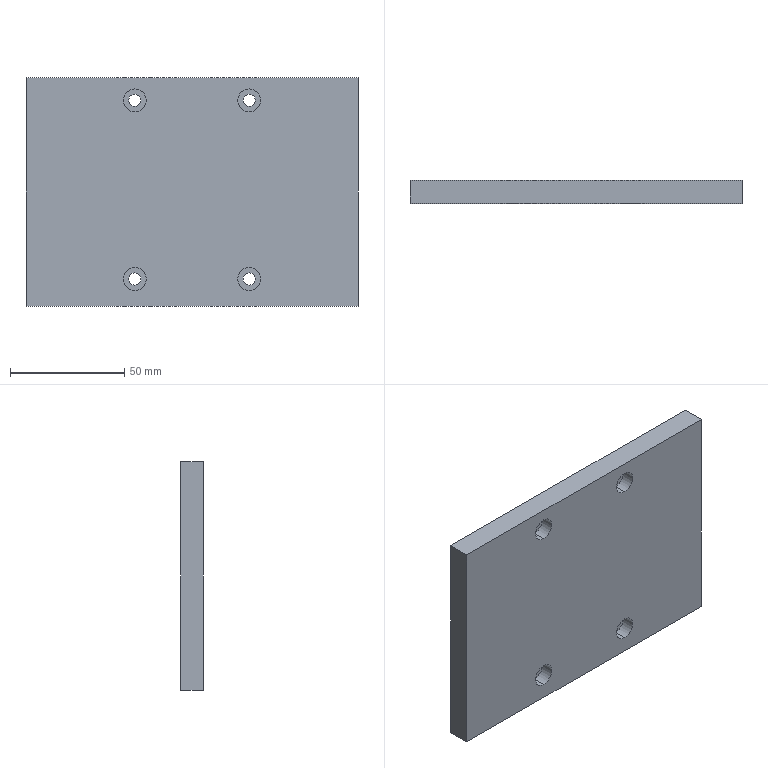Part | SolidWorks | features BaseBody 1 | 1 solid | 26 faces | box 145 x 10 x 100 mm | volume 142830 mm3 | cylinder 16 | plane 10 | commonest cylinder face diameters 5.3 x8 10 x8
STEP:
#1=CARTESIAN_POINT('',(-152.496,1790.044,-108.85));
#2=VERTEX_POINT('',#1);
#3=CARTESIAN_POINT('',(-152.496,1790.044,-114.15));
#4=VERTEX_POINT('',#3);
#5=CARTESIAN_POINT('',(-152.496,1790.044,-111.5));
#6=DIRECTION('',(0.,-1.,0.));
#7=DIRECTION('',(0.,0.,-1.));
#8=AXIS2_PLACEMENT_3D('',#5,#6,#7);
#9=CIRCLE('',#8,2.65);
#10=EDGE_CURVE('',#2,#4,#9,.T.);
#11=ORIENTED_EDGE('',*,*,#10,.F.);
#12=CARTESIAN_POINT('',(-152.496,1785.744,-108.85));
#13=VERTEX_POINT('',#12);
#14=CARTESIAN_POINT('',(-152.496,1780.044,-108.85));
#15=DIRECTION('',(0.,-1.,0.));
#16=VECTOR('',#15,1000.);
#17=LINE('',#14,#16);
#18=EDGE_CURVE('',#2,#13,#17,.T.);
#19=ORIENTED_EDGE('',*,*,#18,.T.);
#20=CARTESIAN_POINT('',(-152.496,1785.744,-114.15));
#21=VERTEX_POINT('',#20);
#22=CARTESIAN_POINT('',(-152.496,1785.744,-111.5));
#23=DIRECTION('',(0.,1.,0.));
#24=DIRECTION('',(0.,0.,-1.));
#25=AXIS2_PLACEMENT_3D('',#22,#23,#24);
#26=CIRCLE('',#25,2.65);
#27=EDGE_CURVE('',#21,#13,#26,.T.);
#28=ORIENTED_EDGE('',*,*,#27,.F.);
#29=CARTESIAN_POINT('',(-152.496,1780.044,-114.15));
#30=DIRECTION('',(0.,-1.,0.));
#31=VECTOR('',#30,1000.);
#32=LINE('',#29,#31);
#33=EDGE_CURVE('',#4,#21,#32,.T.);
#34=ORIENTED_EDGE('',*,*,#33,.F.);
#35=EDGE_LOOP('',(#11,#19,#28,#34));
#36=FACE_OUTER_BOUND('',#35,.T.);
#37=CARTESIAN_POINT('',(-152.496,1780.044,-111.5));
#38=DIRECTION('',(0.,-1.,0.));
#39=DIRECTION('',(0.,0.,-1.));
#40=AXIS2_PLACEMENT_3D('',#37,#38,#39);
#41=CYLINDRICAL_SURFACE('',#40,2.65);
#42=ADVANCED_FACE('',(#36),#41,.F.);
#43=CARTESIAN_POINT('',(-152.496,1790.044,-30.85));
#44=VERTEX_POINT('',#43);
#45=CARTESIAN_POINT('',(-152.496,1790.044,-36.15));
#46=VERTEX_POINT('',#45);
#47=CARTESIAN_POINT('',(-152.496,1790.044,-33.5));
#48=DIRECTION('',(0.,-1.,0.));
#49=DIRECTION('',(0.,0.,-1.));
#50=AXIS2_PLACEMENT_3D('',#47,#48,#49);
#51=CIRCLE('',#50,2.65);
#52=EDGE_CURVE('',#44,#46,#51,.T.);
#53=ORIENTED_EDGE('',*,*,#52,.F.);
#54=CARTESIAN_POINT('',(-152.496,1785.744,-30.85));
#55=VERTEX_POINT('',#54);
#56=CARTESIAN_POINT('',(-152.496,1780.044,-30.85));
#57=DIRECTION('',(0.,-1.,0.));
#58=VECTOR('',#57,1000.);
#59=LINE('',#56,#58);
#60=EDGE_CURVE('',#44,#55,#59,.T.);
#61=ORIENTED_EDGE('',*,*,#60,.T.);
#62=CARTESIAN_POINT('',(-152.496,1785.744,-36.15));
#63=VERTEX_POINT('',#62);
#64=CARTESIAN_POINT('',(-152.496,1785.744,-33.5));
#65=DIRECTION('',(0.,1.,0.));
#66=DIRECTION('',(0.,0.,-1.));
#67=AXIS2_PLACEMENT_3D('',#64,#65,#66);
#68=CIRCLE('',#67,2.65);
#69=EDGE_CURVE('',#63,#55,#68,.T.);
#70=ORIENTED_EDGE('',*,*,#69,.F.);
#71=CARTESIAN_POINT('',(-152.496,1780.044,-36.15));
#72=DIRECTION('',(0.,-1.,0.));
#73=VECTOR('',#72,1000.);
#74=LINE('',#71,#73);
#75=EDGE_CURVE('',#46,#63,#74,.T.);
#76=ORIENTED_EDGE('',*,*,#75,.F.);
#77=EDGE_LOOP('',(#53,#61,#70,#76));
#78=FACE_OUTER_BOUND('',#77,.T.);
#79=CARTESIAN_POINT('',(-152.496,1780.044,-33.5));
#80=DIRECTION('',(0.,-1.,0.));
#81=DIRECTION('',(0.,0.,-1.));
#82=AXIS2_PLACEMENT_3D('',#79,#80,#81);
#83=CYLINDRICAL_SURFACE('',#82,2.65);
#84=ADVANCED_FACE('',(#78),#83,.F.);
#85=CARTESIAN_POINT('',(-102.496,1790.044,-30.85));
#86=VERTEX_POINT('',#85);
#87=CARTESIAN_POINT('',(-102.496,1790.044,-36.15));
#88=VERTEX_POINT('',#87);
#89=CARTESIAN_POINT('',(-102.496,1790.044,-33.5));
#90=DIRECTION('',(0.,-1.,0.));
#91=DIRECTION('',(0.,0.,-1.));
#92=AXIS2_PLACEMENT_3D('',#89,#90,#91);
#93=CIRCLE('',#92,2.65);
#94=EDGE_CURVE('',#86,#88,#93,.T.);
#95=ORIENTED_EDGE('',*,*,#94,.F.);
#96=CARTESIAN_POINT('',(-102.496,1785.744,-30.85));
#97=VERTEX_POINT('',#96);
#98=CARTESIAN_POINT('',(-102.496,1780.044,-30.85));
#99=DIRECTION('',(0.,-1.,0.));
#100=VECTOR('',#99,1000.);
#101=LINE('',#98,#100);
#102=EDGE_CURVE('',#86,#97,#101,.T.);
#103=ORIENTED_EDGE('',*,*,#102,.T.);
#104=CARTESIAN_POINT('',(-102.496,1785.744,-36.15));
#105=VERTEX_POINT('',#104);
#106=CARTESIAN_POINT('',(-102.496,1785.744,-33.5));
#107=DIRECTION('',(0.,1.,0.));
#108=DIRECTION('',(0.,0.,-1.));
#109=AXIS2_PLACEMENT_3D('',#106,#107,#108);
#110=CIRCLE('',#109,2.65);
#111=EDGE_CURVE('',#105,#97,#110,.T.);
#112=ORIENTED_EDGE('',*,*,#111,.F.);
#113=CARTESIAN_POINT('',(-102.496,1780.044,-36.15));
#114=DIRECTION('',(0.,-1.,0.));
#115=VECTOR('',#114,1000.);
#116=LINE('',#113,#115);
#117=EDGE_CURVE('',#88,#105,#116,.T.);
#118=ORIENTED_EDGE('',*,*,#117,.F.);
#119=EDGE_LOOP('',(#95,#103,#112,#118));
#120=FACE_OUTER_BOUND('',#119,.T.);
#121=CARTESIAN_POINT('',(-102.496,1780.044,-33.5));
#122=DIRECTION('',(0.,-1.,0.));
#123=DIRECTION('',(0.,0.,-1.));
#124=AXIS2_PLACEMENT_3D('',#121,#122,#123);
#125=CYLINDRICAL_SURFACE('',#124,2.65);
#126=ADVANCED_FACE('',(#120),#125,.F.);
#127=CARTESIAN_POINT('',(-102.496,1790.044,-108.85));
#128=VERTEX_POINT('',#127);
#129=CARTESIAN_POINT('',(-102.496,1790.044,-114.15));
#130=VERTEX_POINT('',#129);
#131=CARTESIAN_POINT('',(-102.496,1790.044,-111.5));
#132=DIRECTION('',(0.,-1.,0.));
#133=DIRECTION('',(0.,0.,-1.));
#134=AXIS2_PLACEMENT_3D('',#131,#132,#133);
#135=CIRCLE('',#134,2.65);
#136=EDGE_CURVE('',#128,#130,#135,.T.);
#137=ORIENTED_EDGE('',*,*,#136,.F.);
#138=CARTESIAN_POINT('',(-102.496,1785.744,-108.85));
#139=VERTEX_POINT('',#138);
#140=CARTESIAN_POINT('',(-102.496,1780.044,-108.85));
#141=DIRECTION('',(0.,-1.,0.));
#142=VECTOR('',#141,1000.);
#143=LINE('',#140,#142);
#144=EDGE_CURVE('',#128,#139,#143,.T.);
#145=ORIENTED_EDGE('',*,*,#144,.T.);
#146=CARTESIAN_POINT('',(-102.496,1785.744,-114.15));
#147=VERTEX_POINT('',#146);
#148=CARTESIAN_POINT('',(-102.496,1785.744,-111.5));
#149=DIRECTION('',(0.,1.,0.));
#150=DIRECTION('',(0.,0.,-1.));
#151=AXIS2_PLACEMENT_3D('',#148,#149,#150);
#152=CIRCLE('',#151,2.65);
#153=EDGE_CURVE('',#147,#139,#152,.T.);
#154=ORIENTED_EDGE('',*,*,#153,.F.);
#155=CARTESIAN_POINT('',(-102.496,1780.044,-114.15));
#156=DIRECTION('',(0.,-1.,0.));
#157=VECTOR('',#156,1000.);
#158=LINE('',#155,#157);
#159=EDGE_CURVE('',#130,#147,#158,.T.);
#160=ORIENTED_EDGE('',*,*,#159,.F.);
#161=EDGE_LOOP('',(#137,#145,#154,#160));
#162=FACE_OUTER_BOUND('',#161,.T.);
#163=CARTESIAN_POINT('',(-102.496,1780.044,-111.5));
#164=DIRECTION('',(0.,-1.,0.));
#165=DIRECTION('',(0.,0.,-1.));
#166=AXIS2_PLACEMENT_3D('',#163,#164,#165);
#167=CYLINDRICAL_SURFACE('',#166,2.65);
#168=ADVANCED_FACE('',(#162),#167,.F.);
#169=CARTESIAN_POINT('',(-152.496,1785.744,-116.5));
#170=VERTEX_POINT('',#169);
#171=CARTESIAN_POINT('',(-152.496,1785.744,-106.5));
#172=VERTEX_POINT('',#171);
#173=CARTESIAN_POINT('',(-152.496,1785.744,-111.5));
#174=DIRECTION('',(0.,1.,0.));
#175=DIRECTION('',(0.,0.,-1.));
#176=AXIS2_PLACEMENT_3D('',#173,#174,#175);
#177=CIRCLE('',#176,5.);
#178=EDGE_CURVE('',#170,#172,#177,.T.);
#179=ORIENTED_EDGE('',*,*,#178,.T.);
#180=CARTESIAN_POINT('',(-152.496,1780.044,-106.5));
#181=VERTEX_POINT('',#180);
#182=CARTESIAN_POINT('',(-152.496,1780.044,-106.5));
#183=DIRECTION('',(0.,-1.,0.));
#184=VECTOR('',#183,1000.);
#185=LINE('',#182,#184);
#186=EDGE_CURVE('',#172,#181,#185,.T.);
#187=ORIENTED_EDGE('',*,*,#186,.T.);
#188=CARTESIAN_POINT('',(-152.496,1780.044,-116.5));
#189=VERTEX_POINT('',#188);
#190=CARTESIAN_POINT('',(-152.496,1780.044,-111.5));
#191=DIRECTION('',(0.,-1.,0.));
#192=DIRECTION('',(0.,0.,-1.));
#193=AXIS2_PLACEMENT_3D('',#190,#191,#192);
#194=CIRCLE('',#193,5.);
#195=EDGE_CURVE('',#181,#189,#194,.T.);
#196=ORIENTED_EDGE('',*,*,#195,.T.);
#197=CARTESIAN_POINT('',(-152.496,1780.044,-116.5));
#198=DIRECTION('',(0.,-1.,0.));
#199=VECTOR('',#198,1000.);
#200=LINE('',#197,#199);
#201=EDGE_CURVE('',#170,#189,#200,.T.);
#202=ORIENTED_EDGE('',*,*,#201,.F.);
#203=EDGE_LOOP('',(#179,#187,#196,#202));
#204=FACE_OUTER_BOUND('',#203,.T.);
#205=CARTESIAN_POINT('',(-152.496,1780.044,-111.5));
#206=DIRECTION('',(0.,-1.,0.));
#207=DIRECTION('',(0.,0.,-1.));
#208=AXIS2_PLACEMENT_3D('',#205,#206,#207);
#209=CYLINDRICAL_SURFACE('',#208,5.);
#210=ADVANCED_FACE('',(#204),#209,.F.);
#211=CARTESIAN_POINT('',(-152.496,1785.744,-38.5));
#212=VERTEX_POINT('',#211);
#213=CARTESIAN_POINT('',(-152.496,1785.744,-28.5));
#214=VERTEX_POINT('',#213);
#215=CARTESIAN_POINT('',(-152.496,1785.744,-33.5));
#216=DIRECTION('',(0.,1.,0.));
#217=DIRECTION('',(0.,0.,-1.));
#218=AXIS2_PLACEMENT_3D('',#215,#216,#217);
#219=CIRCLE('',#218,5.);
#220=EDGE_CURVE('',#212,#214,#219,.T.);
#221=ORIENTED_EDGE('',*,*,#220,.T.);
#222=CARTESIAN_POINT('',(-152.496,1780.044,-28.5));
#223=VERTEX_POINT('',#222);
#224=CARTESIAN_POINT('',(-152.496,1780.044,-28.5));
#225=DIRECTION('',(0.,-1.,0.));
#226=VECTOR('',#225,1000.);
#227=LINE('',#224,#226);
#228=EDGE_CURVE('',#214,#223,#227,.T.);
#229=ORIENTED_EDGE('',*,*,#228,.T.);
#230=CARTESIAN_POINT('',(-152.496,1780.044,-38.5));
#231=VERTEX_POINT('',#230);
#232=CARTESIAN_POINT('',(-152.496,1780.044,-33.5));
#233=DIRECTION('',(0.,-1.,0.));
#234=DIRECTION('',(0.,0.,-1.));
#235=AXIS2_PLACEMENT_3D('',#232,#233,#234);
#236=CIRCLE('',#235,5.);
#237=EDGE_CURVE('',#223,#231,#236,.T.);
#238=ORIENTED_EDGE('',*,*,#237,.T.);
#239=CARTESIAN_POINT('',(-152.496,1780.044,-38.5));
#240=DIRECTION('',(0.,-1.,0.));
#241=VECTOR('',#240,1000.);
#242=LINE('',#239,#241);
#243=EDGE_CURVE('',#212,#231,#242,.T.);
#244=ORIENTED_EDGE('',*,*,#243,.F.);
#245=EDGE_LOOP('',(#221,#229,#238,#244));
#246=FACE_OUTER_BOUND('',#245,.T.);
#247=CARTESIAN_POINT('',(-152.496,1780.044,-33.5));
#248=DIRECTION('',(0.,-1.,0.));
#249=DIRECTION('',(0.,0.,-1.));
#250=AXIS2_PLACEMENT_3D('',#247,#248,#249);
#251=CYLINDRICAL_SURFACE('',#250,5.);
#252=ADVANCED_FACE('',(#246),#251,.F.);
#253=CARTESIAN_POINT('',(-102.496,1785.744,-38.5));
#254=VERTEX_POINT('',#253);
#255=CARTESIAN_POINT('',(-102.496,1785.744,-28.5));
#256=VERTEX_POINT('',#255);
#257=CARTESIAN_POINT('',(-102.496,1785.744,-33.5));
#258=DIRECTION('',(0.,1.,0.));
#259=DIRECTION('',(0.,0.,-1.));
#260=AXIS2_PLACEMENT_3D('',#257,#258,#259);
#261=CIRCLE('',#260,5.);
#262=EDGE_CURVE('',#254,#256,#261,.T.);
#263=ORIENTED_EDGE('',*,*,#262,.T.);
#264=CARTESIAN_POINT('',(-102.496,1780.044,-28.5));
#265=VERTEX_POINT('',#264);
#266=CARTESIAN_POINT('',(-102.496,1780.044,-28.5));
#267=DIRECTION('',(0.,-1.,0.));
#268=VECTOR('',#267,1000.);
#269=LINE('',#266,#268);
#270=EDGE_CURVE('',#256,#265,#269,.T.);
#271=ORIENTED_EDGE('',*,*,#270,.T.);
#272=CARTESIAN_POINT('',(-102.496,1780.044,-38.5));
#273=VERTEX_POINT('',#272);
#274=CARTESIAN_POINT('',(-102.496,1780.044,-33.5));
#275=DIRECTION('',(0.,-1.,0.));
#276=DIRECTION('',(0.,0.,-1.));
#277=AXIS2_PLACEMENT_3D('',#274,#275,#276);
#278=CIRCLE('',#277,5.);
#279=EDGE_CURVE('',#265,#273,#278,.T.);
#280=ORIENTED_EDGE('',*,*,#279,.T.);
#281=CARTESIAN_POINT('',(-102.496,1780.044,-38.5));
#282=DIRECTION('',(0.,-1.,0.));
#283=VECTOR('',#282,1000.);
#284=LINE('',#281,#283);
#285=EDGE_CURVE('',#254,#273,#284,.T.);
#286=ORIENTED_EDGE('',*,*,#285,.F.);
#287=EDGE_LOOP('',(#263,#271,#280,#286));
#288=FACE_OUTER_BOUND('',#287,.T.);
#289=CARTESIAN_POINT('',(-102.496,1780.044,-33.5));
#290=DIRECTION('',(0.,-1.,0.));
#291=DIRECTION('',(0.,0.,-1.));
#292=AXIS2_PLACEMENT_3D('',#289,#290,#291);
#293=CYLINDRICAL_SURFACE('',#292,5.);
#294=ADVANCED_FACE('',(#288),#293,.F.);
#295=CARTESIAN_POINT('',(-102.496,1785.744,-116.5));
#296=VERTEX_POINT('',#295);
#297=CARTESIAN_POINT('',(-102.496,1785.744,-106.5));
#298=VERTEX_POINT('',#297);
#299=CARTESIAN_POINT('',(-102.496,1785.744,-111.5));
#300=DIRECTION('',(0.,1.,0.));
#301=DIRECTION('',(0.,0.,-1.));
#302=AXIS2_PLACEMENT_3D('',#299,#300,#301);
#303=CIRCLE('',#302,5.);
#304=EDGE_CURVE('',#296,#298,#303,.T.);
#305=ORIENTED_EDGE('',*,*,#304,.T.);
#306=CARTESIAN_POINT('',(-102.496,1780.044,-106.5));
#307=VERTEX_POINT('',#306);
#308=CARTESIAN_POINT('',(-102.496,1780.044,-106.5));
#309=DIRECTION('',(0.,-1.,0.));
#310=VECTOR('',#309,1000.);
#311=LINE('',#308,#310);
#312=EDGE_CURVE('',#298,#307,#311,.T.);
#313=ORIENTED_EDGE('',*,*,#312,.T.);
#314=CARTESIAN_POINT('',(-102.496,1780.044,-116.5));
#315=VERTEX_POINT('',#314);
#316=CARTESIAN_POINT('',(-102.496,1780.044,-111.5));
#317=DIRECTION('',(0.,-1.,0.));
#318=DIRECTION('',(0.,0.,-1.));
#319=AXIS2_PLACEMENT_3D('',#316,#317,#318);
#320=CIRCLE('',#319,5.);
#321=EDGE_CURVE('',#307,#315,#320,.T.);
#322=ORIENTED_EDGE('',*,*,#321,.T.);
#323=CARTESIAN_POINT('',(-102.496,1780.044,-116.5));
#324=DIRECTION('',(0.,-1.,0.));
#325=VECTOR('',#324,1000.);
#326=LINE('',#323,#325);
#327=EDGE_CURVE('',#296,#315,#326,.T.);
#328=ORIENTED_EDGE('',*,*,#327,.F.);
#329=EDGE_LOOP('',(#305,#313,#322,#328));
#330=FACE_OUTER_BOUND('',#329,.T.);
#331=CARTESIAN_POINT('',(-102.496,1780.044,-111.5));
#332=DIRECTION('',(0.,-1.,0.));
#333=DIRECTION('',(0.,0.,-1.));
#334=AXIS2_PLACEMENT_3D('',#331,#332,#333);
#335=CYLINDRICAL_SURFACE('',#334,5.);
#336=ADVANCED_FACE('',(#330),#335,.F.);
#337=CARTESIAN_POINT('',(-152.496,1790.044,-111.5));
#338=DIRECTION('',(0.,-1.,0.));
#339=DIRECTION('',(0.,0.,-1.));
#340=AXIS2_PLACEMENT_3D('',#337,#338,#339);
#341=CIRCLE('',#340,2.65);
#342=EDGE_CURVE('',#4,#2,#341,.T.);
#343=ORIENTED_EDGE('',*,*,#342,.T.);
#344=ORIENTED_EDGE('',*,*,#10,.T.);
#345=EDGE_LOOP('',(#343,#344));
#346=FACE_BOUND('',#345,.T.);
#347=CARTESIAN_POINT('',(-152.496,1790.044,-33.5));
#348=DIRECTION('',(0.,-1.,0.));
#349=DIRECTION('',(0.,0.,-1.));
#350=AXIS2_PLACEMENT_3D('',#347,#348,#349);
#351=CIRCLE('',#350,2.65);
#352=EDGE_CURVE('',#46,#44,#351,.T.);
#353=ORIENTED_EDGE('',*,*,#352,.T.);
#354=ORIENTED_EDGE('',*,*,#52,.T.);
#355=EDGE_LOOP('',(#353,#354));
#356=FACE_BOUND('',#355,.T.);
#357=CARTESIAN_POINT('',(-102.496,1790.044,-33.5));
#358=DIRECTION('',(0.,-1.,0.));
#359=DIRECTION('',(0.,0.,-1.));
#360=AXIS2_PLACEMENT_3D('',#357,#358,#359);
#361=CIRCLE('',#360,2.65);
#362=EDGE_CURVE('',#88,#86,#361,.T.);
#363=ORIENTED_EDGE('',*,*,#362,.T.);
#364=ORIENTED_EDGE('',*,*,#94,.T.);
#365=EDGE_LOOP('',(#363,#364));
#366=FACE_BOUND('',#365,.T.);
#367=CARTESIAN_POINT('',(-102.496,1790.044,-111.5));
#368=DIRECTION('',(0.,-1.,0.));
#369=DIRECTION('',(0.,0.,-1.));
#370=AXIS2_PLACEMENT_3D('',#367,#368,#369);
#371=CIRCLE('',#370,2.65);
#372=EDGE_CURVE('',#130,#128,#371,.T.);
#373=ORIENTED_EDGE('',*,*,#372,.T.);
#374=ORIENTED_EDGE('',*,*,#136,.T.);
#375=EDGE_LOOP('',(#373,#374));
#376=FACE_BOUND('',#375,.T.);
#377=CARTESIAN_POINT('',(-199.996,1790.044,-123.5));
#378=VERTEX_POINT('',#377);
#379=CARTESIAN_POINT('',(-199.996,1790.044,-23.5));
#380=VERTEX_POINT('',#379);
#381=CARTESIAN_POINT('',(-199.996,1790.044,-123.5));
#382=DIRECTION('',(0.,0.,1.));
#383=VECTOR('',#382,1000.);
#384=LINE('',#381,#383);
#385=EDGE_CURVE('',#378,#380,#384,.T.);
#386=ORIENTED_EDGE('',*,*,#385,.T.);
#387=CARTESIAN_POINT('',(-54.996,1790.044,-23.5));
#388=VERTEX_POINT('',#387);
#389=CARTESIAN_POINT('',(47.504,1790.044,-23.5));
#390=DIRECTION('',(1.,0.,0.));
#391=VECTOR('',#390,1000.);
#392=LINE('',#389,#391);
#393=EDGE_CURVE('',#380,#388,#392,.T.);
#394=ORIENTED_EDGE('',*,*,#393,.T.);
#395=CARTESIAN_POINT('',(-54.996,1790.044,-123.5));
#396=VERTEX_POINT('',#395);
#397=CARTESIAN_POINT('',(-54.996,1790.044,-123.5));
#398=DIRECTION('',(0.,0.,-1.));
#399=VECTOR('',#398,1000.);
#400=LINE('',#397,#399);
#401=EDGE_CURVE('',#388,#396,#400,.T.);
#402=ORIENTED_EDGE('',*,*,#401,.T.);
#403=CARTESIAN_POINT('',(47.504,1790.044,-123.5));
#404=DIRECTION('',(-1.,0.,0.));
#405=VECTOR('',#404,1000.);
#406=LINE('',#403,#405);
#407=EDGE_CURVE('',#396,#378,#406,.T.);
#408=ORIENTED_EDGE('',*,*,#407,.T.);
#409=EDGE_LOOP('',(#386,#394,#402,#408));
#410=FACE_OUTER_BOUND('',#409,.T.);
#411=CARTESIAN_POINT('',(47.504,1790.044,-123.5));
#412=DIRECTION('',(0.,1.,0.));
#413=DIRECTION('',(0.,0.,1.));
#414=AXIS2_PLACEMENT_3D('',#411,#412,#413);
#415=PLANE('',#414);
#416=ADVANCED_FACE('',(#346,#356,#366,#376,#410),#415,.T.);
#417=ORIENTED_EDGE('',*,*,#18,.F.);
#418=ORIENTED_EDGE('',*,*,#342,.F.);
#419=ORIENTED_EDGE('',*,*,#33,.T.);
#420=CARTESIAN_POINT('',(-152.496,1785.744,-111.5));
#421=DIRECTION('',(0.,1.,0.));
#422=DIRECTION('',(0.,0.,-1.));
#423=AXIS2_PLACEMENT_3D('',#420,#421,#422);
#424=CIRCLE('',#423,2.65);
#425=EDGE_CURVE('',#13,#21,#424,.T.);
#426=ORIENTED_EDGE('',*,*,#425,.F.);
#427=EDGE_LOOP('',(#417,#418,#419,#426));
#428=FACE_OUTER_BOUND('',#427,.T.);
#429=CARTESIAN_POINT('',(-152.496,1780.044,-111.5));
#430=DIRECTION('',(0.,-1.,0.));
#431=DIRECTION('',(0.,0.,-1.));
#432=AXIS2_PLACEMENT_3D('',#429,#430,#431);
#433=CYLINDRICAL_SURFACE('',#432,2.65);
#434=ADVANCED_FACE('',(#428),#433,.F.);
#435=ORIENTED_EDGE('',*,*,#60,.F.);
#436=ORIENTED_EDGE('',*,*,#352,.F.);
#437=ORIENTED_EDGE('',*,*,#75,.T.);
#438=CARTESIAN_POINT('',(-152.496,1785.744,-33.5));
#439=DIRECTION('',(0.,1.,0.));
#440=DIRECTION('',(0.,0.,-1.));
#441=AXIS2_PLACEMENT_3D('',#438,#439,#440);
#442=CIRCLE('',#441,2.65);
#443=EDGE_CURVE('',#55,#63,#442,.T.);
#444=ORIENTED_EDGE('',*,*,#443,.F.);
#445=EDGE_LOOP('',(#435,#436,#437,#444));
#446=FACE_OUTER_BOUND('',#445,.T.);
#447=CARTESIAN_POINT('',(-152.496,1780.044,-33.5));
#448=DIRECTION('',(0.,-1.,0.));
#449=DIRECTION('',(0.,0.,-1.));
#450=AXIS2_PLACEMENT_3D('',#447,#448,#449);
#451=CYLINDRICAL_SURFACE('',#450,2.65);
#452=ADVANCED_FACE('',(#446),#451,.F.);
#453=ORIENTED_EDGE('',*,*,#102,.F.);
#454=ORIENTED_EDGE('',*,*,#362,.F.);
#455=ORIENTED_EDGE('',*,*,#117,.T.);
#456=CARTESIAN_POINT('',(-102.496,1785.744,-33.5));
#457=DIRECTION('',(0.,1.,0.));
#458=DIRECTION('',(0.,0.,-1.));
#459=AXIS2_PLACEMENT_3D('',#456,#457,#458);
#460=CIRCLE('',#459,2.65);
#461=EDGE_CURVE('',#97,#105,#460,.T.);
#462=ORIENTED_EDGE('',*,*,#461,.F.);
#463=EDGE_LOOP('',(#453,#454,#455,#462));
#464=FACE_OUTER_BOUND('',#463,.T.);
#465=CARTESIAN_POINT('',(-102.496,1780.044,-33.5));
#466=DIRECTION('',(0.,-1.,0.));
#467=DIRECTION('',(0.,0.,-1.));
#468=AXIS2_PLACEMENT_3D('',#465,#466,#467);
#469=CYLINDRICAL_SURFACE('',#468,2.65);
#470=ADVANCED_FACE('',(#464),#469,.F.);
#471=ORIENTED_EDGE('',*,*,#144,.F.);
#472=ORIENTED_EDGE('',*,*,#372,.F.);
#473=ORIENTED_EDGE('',*,*,#159,.T.);
#474=CARTESIAN_POINT('',(-102.496,1785.744,-111.5));
#475=DIRECTION('',(0.,1.,0.));
#476=DIRECTION('',(0.,0.,-1.));
#477=AXIS2_PLACEMENT_3D('',#474,#475,#476);
#478=CIRCLE('',#477,2.65);
#479=EDGE_CURVE('',#139,#147,#478,.T.);
#480=ORIENTED_EDGE('',*,*,#479,.F.);
#481=EDGE_LOOP('',(#471,#472,#473,#480));
#482=FACE_OUTER_BOUND('',#481,.T.);
#483=CARTESIAN_POINT('',(-102.496,1780.044,-111.5));
#484=DIRECTION('',(0.,-1.,0.));
#485=DIRECTION('',(0.,0.,-1.));
#486=AXIS2_PLACEMENT_3D('',#483,#484,#485);
#487=CYLINDRICAL_SURFACE('',#486,2.65);
#488=ADVANCED_FACE('',(#482),#487,.F.);
#489=ORIENTED_EDGE('',*,*,#393,.F.);
#490=CARTESIAN_POINT('',(-199.996,1780.044,-23.5));
#491=VERTEX_POINT('',#490);
#492=CARTESIAN_POINT('',(-199.996,1790.044,-23.5));
#493=DIRECTION('',(0.,1.,0.));
#494=VECTOR('',#493,1000.);
#495=LINE('',#492,#494);
#496=EDGE_CURVE('',#491,#380,#495,.T.);
#497=ORIENTED_EDGE('',*,*,#496,.F.);
#498=CARTESIAN_POINT('',(-54.996,1780.044,-23.5));
#499=VERTEX_POINT('',#498);
#500=CARTESIAN_POINT('',(47.504,1780.044,-23.5));
#501=DIRECTION('',(-1.,0.,0.));
#502=VECTOR('',#501,1000.);
#503=LINE('',#500,#502);
#504=EDGE_CURVE('',#499,#491,#503,.T.);
#505=ORIENTED_EDGE('',*,*,#504,.F.);
#506=CARTESIAN_POINT('',(-54.996,1790.044,-23.5));
#507=DIRECTION('',(0.,-1.,0.));
#508=VECTOR('',#507,1000.);
#509=LINE('',#506,#508);
#510=EDGE_CURVE('',#388,#499,#509,.T.);
#511=ORIENTED_EDGE('',*,*,#510,.F.);
#512=EDGE_LOOP('',(#489,#497,#505,#511));
#513=FACE_OUTER_BOUND('',#512,.T.);
#514=CARTESIAN_POINT('',(47.504,1790.044,-23.5));
#515=DIRECTION('',(0.,0.,-1.));
#516=DIRECTION('',(-1.,0.,0.));
#517=AXIS2_PLACEMENT_3D('',#514,#515,#516);
#518=PLANE('',#517);
#519=ADVANCED_FACE('',(#513),#518,.F.);
#520=CARTESIAN_POINT('',(-199.996,1780.044,-123.5));
#521=VERTEX_POINT('',#520);
#522=CARTESIAN_POINT('',(-199.996,1780.044,-100.5));
#523=DIRECTION('',(0.,0.,-1.));
#524=VECTOR('',#523,1000.);
#525=LINE('',#522,#524);
#526=EDGE_CURVE('',#491,#521,#525,.T.);
#527=ORIENTED_EDGE('',*,*,#526,.F.);
#528=ORIENTED_EDGE('',*,*,#496,.T.);
#529=ORIENTED_EDGE('',*,*,#385,.F.);
#530=CARTESIAN_POINT('',(-199.996,1790.044,-123.5));
#531=DIRECTION('',(0.,1.,0.));
#532=VECTOR('',#531,1000.);
#533=LINE('',#530,#532);
#534=EDGE_CURVE('',#521,#378,#533,.T.);
#535=ORIENTED_EDGE('',*,*,#534,.F.);
#536=EDGE_LOOP('',(#527,#528,#529,#535));
#537=FACE_OUTER_BOUND('',#536,.T.);
#538=CARTESIAN_POINT('',(-199.996,1790.044,-100.5));
#539=DIRECTION('',(1.,0.,0.));
#540=DIRECTION('',(0.,0.,-1.));
#541=AXIS2_PLACEMENT_3D('',#538,#539,#540);
#542=PLANE('',#541);
#543=ADVANCED_FACE('',(#537),#542,.F.);
#544=ORIENTED_EDGE('',*,*,#407,.F.);
#545=CARTESIAN_POINT('',(-54.996,1780.044,-123.5));
#546=VERTEX_POINT('',#545);
#547=CARTESIAN_POINT('',(-54.996,1790.044,-123.5));
#548=DIRECTION('',(0.,1.,0.));
#549=VECTOR('',#548,1000.);
#550=LINE('',#547,#549);
#551=EDGE_CURVE('',#546,#396,#550,.T.);
#552=ORIENTED_EDGE('',*,*,#551,.F.);
#553=CARTESIAN_POINT('',(47.504,1780.044,-123.5));
#554=DIRECTION('',(1.,0.,0.));
#555=VECTOR('',#554,1000.);
#556=LINE('',#553,#555);
#557=EDGE_CURVE('',#521,#546,#556,.T.);
#558=ORIENTED_EDGE('',*,*,#557,.F.);
#559=ORIENTED_EDGE('',*,*,#534,.T.);
#560=EDGE_LOOP('',(#544,#552,#558,#559));
#561=FACE_OUTER_BOUND('',#560,.T.);
#562=CARTESIAN_POINT('',(47.504,1790.044,-123.5));
#563=DIRECTION('',(0.,0.,1.));
#564=DIRECTION('',(1.,0.,0.));
#565=AXIS2_PLACEMENT_3D('',#562,#563,#564);
#566=PLANE('',#565);
#567=ADVANCED_FACE('',(#561),#566,.F.);
#568=ORIENTED_EDGE('',*,*,#510,.T.);
#569=CARTESIAN_POINT('',(-54.996,1780.044,-100.5));
#570=DIRECTION('',(0.,0.,1.));
#571=VECTOR('',#570,1000.);
#572=LINE('',#569,#571);
#573=EDGE_CURVE('',#546,#499,#572,.T.);
#574=ORIENTED_EDGE('',*,*,#573,.F.);
#575=ORIENTED_EDGE('',*,*,#551,.T.);
#576=ORIENTED_EDGE('',*,*,#401,.F.);
#577=EDGE_LOOP('',(#568,#574,#575,#576));
#578=FACE_OUTER_BOUND('',#577,.T.);
#579=CARTESIAN_POINT('',(-54.996,1790.044,-100.5));
#580=DIRECTION('',(-1.,0.,0.));
#581=DIRECTION('',(0.,0.,1.));
#582=AXIS2_PLACEMENT_3D('',#579,#580,#581);
#583=PLANE('',#582);
#584=ADVANCED_FACE('',(#578),#583,.F.);
#585=ORIENTED_EDGE('',*,*,#27,.T.);
#586=ORIENTED_EDGE('',*,*,#425,.T.);
#587=EDGE_LOOP('',(#585,#586));
#588=FACE_BOUND('',#587,.T.);
#589=ORIENTED_EDGE('',*,*,#178,.F.);
#590=CARTESIAN_POINT('',(-152.496,1785.744,-111.5));
#591=DIRECTION('',(0.,1.,0.));
#592=DIRECTION('',(0.,0.,-1.));
#593=AXIS2_PLACEMENT_3D('',#590,#591,#592);
#594=CIRCLE('',#593,5.);
#595=EDGE_CURVE('',#172,#170,#594,.T.);
#596=ORIENTED_EDGE('',*,*,#595,.F.);
#597=EDGE_LOOP('',(#589,#596));
#598=FACE_OUTER_BOUND('',#597,.T.);
#599=CARTESIAN_POINT('',(-155.146,1785.744,-111.5));
#600=DIRECTION('',(0.,1.,0.));
#601=DIRECTION('',(0.,0.,1.));
#602=AXIS2_PLACEMENT_3D('',#599,#600,#601);
#603=PLANE('',#602);
#604=ADVANCED_FACE('',(#588,#598),#603,.F.);
#605=ORIENTED_EDGE('',*,*,#69,.T.);
#606=ORIENTED_EDGE('',*,*,#443,.T.);
#607=EDGE_LOOP('',(#605,#606));
#608=FACE_BOUND('',#607,.T.);
#609=ORIENTED_EDGE('',*,*,#220,.F.);
#610=CARTESIAN_POINT('',(-152.496,1785.744,-33.5));
#611=DIRECTION('',(0.,1.,0.));
#612=DIRECTION('',(0.,0.,-1.));
#613=AXIS2_PLACEMENT_3D('',#610,#611,#612);
#614=CIRCLE('',#613,5.);
#615=EDGE_CURVE('',#214,#212,#614,.T.);
#616=ORIENTED_EDGE('',*,*,#615,.F.);
#617=EDGE_LOOP('',(#609,#616));
#618=FACE_OUTER_BOUND('',#617,.T.);
#619=CARTESIAN_POINT('',(-155.146,1785.744,-33.5));
#620=DIRECTION('',(0.,1.,0.));
#621=DIRECTION('',(0.,0.,1.));
#622=AXIS2_PLACEMENT_3D('',#619,#620,#621);
#623=PLANE('',#622);
#624=ADVANCED_FACE('',(#608,#618),#623,.F.);
#625=ORIENTED_EDGE('',*,*,#111,.T.);
#626=ORIENTED_EDGE('',*,*,#461,.T.);
#627=EDGE_LOOP('',(#625,#626));
#628=FACE_BOUND('',#627,.T.);
#629=ORIENTED_EDGE('',*,*,#262,.F.);
#630=CARTESIAN_POINT('',(-102.496,1785.744,-33.5));
#631=DIRECTION('',(0.,1.,0.));
#632=DIRECTION('',(0.,0.,-1.));
#633=AXIS2_PLACEMENT_3D('',#630,#631,#632);
#634=CIRCLE('',#633,5.);
#635=EDGE_CURVE('',#256,#254,#634,.T.);
#636=ORIENTED_EDGE('',*,*,#635,.F.);
#637=EDGE_LOOP('',(#629,#636));
#638=FACE_OUTER_BOUND('',#637,.T.);
#639=CARTESIAN_POINT('',(-105.146,1785.744,-33.5));
#640=DIRECTION('',(0.,1.,0.));
#641=DIRECTION('',(0.,0.,1.));
#642=AXIS2_PLACEMENT_3D('',#639,#640,#641);
#643=PLANE('',#642);
#644=ADVANCED_FACE('',(#628,#638),#643,.F.);
#645=ORIENTED_EDGE('',*,*,#153,.T.);
#646=ORIENTED_EDGE('',*,*,#479,.T.);
#647=EDGE_LOOP('',(#645,#646));
#648=FACE_BOUND('',#647,.T.);
#649=ORIENTED_EDGE('',*,*,#304,.F.);
#650=CARTESIAN_POINT('',(-102.496,1785.744,-111.5));
#651=DIRECTION('',(0.,1.,0.));
#652=DIRECTION('',(0.,0.,-1.));
#653=AXIS2_PLACEMENT_3D('',#650,#651,#652);
#654=CIRCLE('',#653,5.);
#655=EDGE_CURVE('',#298,#296,#654,.T.);
#656=ORIENTED_EDGE('',*,*,#655,.F.);
#657=EDGE_LOOP('',(#649,#656));
#658=FACE_OUTER_BOUND('',#657,.T.);
#659=CARTESIAN_POINT('',(-105.146,1785.744,-111.5));
#660=DIRECTION('',(0.,1.,0.));
#661=DIRECTION('',(0.,0.,1.));
#662=AXIS2_PLACEMENT_3D('',#659,#660,#661);
#663=PLANE('',#662);
#664=ADVANCED_FACE('',(#648,#658),#663,.F.);
#665=CARTESIAN_POINT('',(-152.496,1780.044,-111.5));
#666=DIRECTION('',(0.,-1.,0.));
#667=DIRECTION('',(0.,0.,-1.));
#668=AXIS2_PLACEMENT_3D('',#665,#666,#667);
#669=CIRCLE('',#668,5.);
#670=EDGE_CURVE('',#189,#181,#669,.T.);
#671=ORIENTED_EDGE('',*,*,#670,.F.);
#672=ORIENTED_EDGE('',*,*,#195,.F.);
#673=EDGE_LOOP('',(#671,#672));
#674=FACE_BOUND('',#673,.T.);
#675=CARTESIAN_POINT('',(-152.496,1780.044,-33.5));
#676=DIRECTION('',(0.,-1.,0.));
#677=DIRECTION('',(0.,0.,-1.));
#678=AXIS2_PLACEMENT_3D('',#675,#676,#677);
#679=CIRCLE('',#678,5.);
#680=EDGE_CURVE('',#231,#223,#679,.T.);
#681=ORIENTED_EDGE('',*,*,#680,.F.);
#682=ORIENTED_EDGE('',*,*,#237,.F.);
#683=EDGE_LOOP('',(#681,#682));
#684=FACE_BOUND('',#683,.T.);
#685=CARTESIAN_POINT('',(-102.496,1780.044,-33.5));
#686=DIRECTION('',(0.,-1.,0.));
#687=DIRECTION('',(0.,0.,-1.));
#688=AXIS2_PLACEMENT_3D('',#685,#686,#687);
#689=CIRCLE('',#688,5.);
#690=EDGE_CURVE('',#273,#265,#689,.T.);
#691=ORIENTED_EDGE('',*,*,#690,.F.);
#692=ORIENTED_EDGE('',*,*,#279,.F.);
#693=EDGE_LOOP('',(#691,#692));
#694=FACE_BOUND('',#693,.T.);
#695=CARTESIAN_POINT('',(-102.496,1780.044,-111.5));
#696=DIRECTION('',(0.,-1.,0.));
#697=DIRECTION('',(0.,0.,-1.));
#698=AXIS2_PLACEMENT_3D('',#695,#696,#697);
#699=CIRCLE('',#698,5.);
#700=EDGE_CURVE('',#315,#307,#699,.T.);
#701=ORIENTED_EDGE('',*,*,#700,.F.);
#702=ORIENTED_EDGE('',*,*,#321,.F.);
#703=EDGE_LOOP('',(#701,#702));
#704=FACE_BOUND('',#703,.T.);
#705=ORIENTED_EDGE('',*,*,#504,.T.);
#706=ORIENTED_EDGE('',*,*,#526,.T.);
#707=ORIENTED_EDGE('',*,*,#557,.T.);
#708=ORIENTED_EDGE('',*,*,#573,.T.);
#709=EDGE_LOOP('',(#705,#706,#707,#708));
#710=FACE_OUTER_BOUND('',#709,.T.);
#711=CARTESIAN_POINT('',(47.504,1780.044,-123.5));
#712=DIRECTION('',(0.,1.,0.));
#713=DIRECTION('',(0.,0.,1.));
#714=AXIS2_PLACEMENT_3D('',#711,#712,#713);
#715=PLANE('',#714);
#716=ADVANCED_FACE('',(#674,#684,#694,#704,#710),#715,.F.);
#717=ORIENTED_EDGE('',*,*,#186,.F.);
#718=ORIENTED_EDGE('',*,*,#595,.T.);
#719=ORIENTED_EDGE('',*,*,#201,.T.);
#720=ORIENTED_EDGE('',*,*,#670,.T.);
#721=EDGE_LOOP('',(#717,#718,#719,#720));
#722=FACE_OUTER_BOUND('',#721,.T.);
#723=CARTESIAN_POINT('',(-152.496,1780.044,-111.5));
#724=DIRECTION('',(0.,-1.,0.));
#725=DIRECTION('',(0.,0.,-1.));
#726=AXIS2_PLACEMENT_3D('',#723,#724,#725);
#727=CYLINDRICAL_SURFACE('',#726,5.);
#728=ADVANCED_FACE('',(#722),#727,.F.);
#729=ORIENTED_EDGE('',*,*,#228,.F.);
#730=ORIENTED_EDGE('',*,*,#615,.T.);
#731=ORIENTED_EDGE('',*,*,#243,.T.);
#732=ORIENTED_EDGE('',*,*,#680,.T.);
#733=EDGE_LOOP('',(#729,#730,#731,#732));
#734=FACE_OUTER_BOUND('',#733,.T.);
#735=CARTESIAN_POINT('',(-152.496,1780.044,-33.5));
#736=DIRECTION('',(0.,-1.,0.));
#737=DIRECTION('',(0.,0.,-1.));
#738=AXIS2_PLACEMENT_3D('',#735,#736,#737);
#739=CYLINDRICAL_SURFACE('',#738,5.);
#740=ADVANCED_FACE('',(#734),#739,.F.);
#741=ORIENTED_EDGE('',*,*,#270,.F.);
#742=ORIENTED_EDGE('',*,*,#635,.T.);
#743=ORIENTED_EDGE('',*,*,#285,.T.);
#744=ORIENTED_EDGE('',*,*,#690,.T.);
#745=EDGE_LOOP('',(#741,#742,#743,#744));
#746=FACE_OUTER_BOUND('',#745,.T.);
#747=CARTESIAN_POINT('',(-102.496,1780.044,-33.5));
#748=DIRECTION('',(0.,-1.,0.));
#749=DIRECTION('',(0.,0.,-1.));
#750=AXIS2_PLACEMENT_3D('',#747,#748,#749);
#751=CYLINDRICAL_SURFACE('',#750,5.);
#752=ADVANCED_FACE('',(#746),#751,.F.);
#753=ORIENTED_EDGE('',*,*,#312,.F.);
#754=ORIENTED_EDGE('',*,*,#655,.T.);
#755=ORIENTED_EDGE('',*,*,#327,.T.);
#756=ORIENTED_EDGE('',*,*,#700,.T.);
#757=EDGE_LOOP('',(#753,#754,#755,#756));
#758=FACE_OUTER_BOUND('',#757,.T.);
#759=CARTESIAN_POINT('',(-102.496,1780.044,-111.5));
#760=DIRECTION('',(0.,-1.,0.));
#761=DIRECTION('',(0.,0.,-1.));
#762=AXIS2_PLACEMENT_3D('',#759,#760,#761);
#763=CYLINDRICAL_SURFACE('',#762,5.);
#764=ADVANCED_FACE('',(#758),#763,.F.);
#765=CLOSED_SHELL('',(#42,#84,#126,#168,#210,#252,#294,#336,#416,#434,#452,#470,#488,#519,#543,#567,#584,#604,#624,#644,#664,#716,#728,#740,#752,#764));
#766=MANIFOLD_SOLID_BREP('',#765);
#767=CARTESIAN_POINT('',(0.,0.,0.));
#768=DIRECTION('',(0.,0.,1.));
#769=DIRECTION('',(1.,0.,0.));
#770=AXIS2_PLACEMENT_3D('',#767,#768,#769);
#771=(LENGTH_UNIT()NAMED_UNIT(*)SI_UNIT(.MILLI.,.METRE.));
#772=UNCERTAINTY_MEASURE_WITH_UNIT(LENGTH_MEASURE(0.00001),#771,'','');
#773=(NAMED_UNIT(*)PLANE_ANGLE_UNIT()SI_UNIT($,.RADIAN.));
#774=(NAMED_UNIT(*)SI_UNIT($,.STERADIAN.)SOLID_ANGLE_UNIT());
#775=(GEOMETRIC_REPRESENTATION_CONTEXT(3)GLOBAL_UNCERTAINTY_ASSIGNED_CONTEXT((#772))GLOBAL_UNIT_ASSIGNED_CONTEXT((#771,#773,#774))REPRESENTATION_CONTEXT('',''));
#776=ADVANCED_BREP_SHAPE_REPRESENTATION('',(#766,#770),#775);